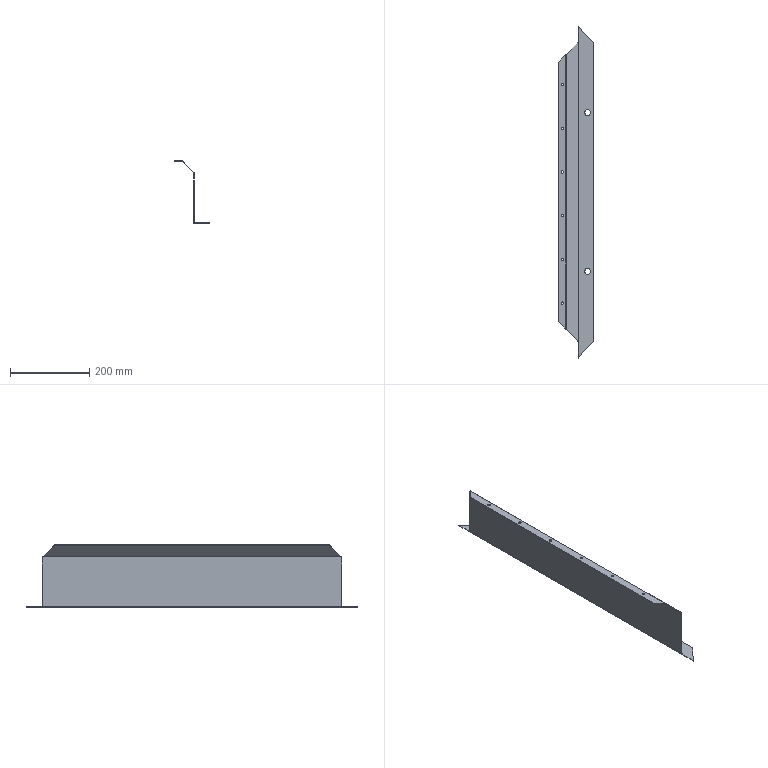Part | NX | features solid 2 | 1 solid | 52 faces | box 88.8 x 836 x 158 mm | volume 203156 mm3 | plane 26 | cylinder 22 | spline 4 | commonest cylinder face diameters 6 x12 15 x4 2.4 x3 4.8 x3